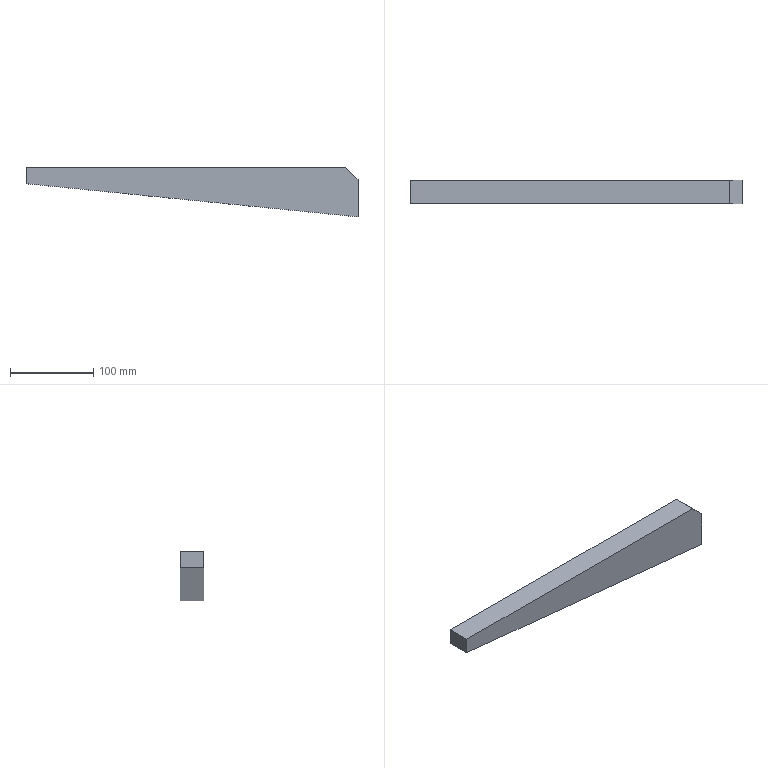Part | SolidWorks | features Extrusion 1 | 1 solid | 7 faces | box 400 x 28 x 60 mm | volume 444850 mm3 | plane 7
STEP:
#1=CARTESIAN_POINT('',(2011.524,0.,-1604.008));
#2=VERTEX_POINT('',#1);
#3=CARTESIAN_POINT('',(2011.524,0.,-1584.008));
#4=VERTEX_POINT('',#3);
#5=CARTESIAN_POINT('',(2011.524,0.,-1604.008));
#6=DIRECTION('',(0.,0.,1.));
#7=VECTOR('',#6,1000.);
#8=LINE('',#5,#7);
#9=EDGE_CURVE('',#2,#4,#8,.T.);
#10=ORIENTED_EDGE('',*,*,#9,.T.);
#11=CARTESIAN_POINT('',(2011.524,28.,-1584.008));
#12=VERTEX_POINT('',#11);
#13=CARTESIAN_POINT('',(2011.524,28.,-1584.008));
#14=DIRECTION('',(0.,-1.,0.));
#15=VECTOR('',#14,1000.);
#16=LINE('',#13,#15);
#17=EDGE_CURVE('',#12,#4,#16,.T.);
#18=ORIENTED_EDGE('',*,*,#17,.F.);
#19=CARTESIAN_POINT('',(2011.524,28.,-1604.008));
#20=VERTEX_POINT('',#19);
#21=CARTESIAN_POINT('',(2011.524,28.,-1604.008));
#22=DIRECTION('',(0.,0.,1.));
#23=VECTOR('',#22,1000.);
#24=LINE('',#21,#23);
#25=EDGE_CURVE('',#20,#12,#24,.T.);
#26=ORIENTED_EDGE('',*,*,#25,.F.);
#27=CARTESIAN_POINT('',(2011.524,28.,-1604.008));
#28=DIRECTION('',(0.,-1.,0.));
#29=VECTOR('',#28,1000.);
#30=LINE('',#27,#29);
#31=EDGE_CURVE('',#20,#2,#30,.T.);
#32=ORIENTED_EDGE('',*,*,#31,.T.);
#33=EDGE_LOOP('',(#10,#18,#26,#32));
#34=FACE_OUTER_BOUND('',#33,.T.);
#35=CARTESIAN_POINT('',(2011.524,28.,-1604.008));
#36=DIRECTION('',(1.,0.,0.));
#37=DIRECTION('',(0.,0.,-1.));
#38=AXIS2_PLACEMENT_3D('',#35,#36,#37);
#39=PLANE('',#38);
#40=ADVANCED_FACE('',(#34),#39,.F.);
#41=CARTESIAN_POINT('',(2396.524,0.,-1584.008));
#42=VERTEX_POINT('',#41);
#43=CARTESIAN_POINT('',(2011.524,0.,-1584.008));
#44=DIRECTION('',(1.,0.,0.));
#45=VECTOR('',#44,1000.);
#46=LINE('',#43,#45);
#47=EDGE_CURVE('',#4,#42,#46,.T.);
#48=ORIENTED_EDGE('',*,*,#47,.T.);
#49=CARTESIAN_POINT('',(2396.524,28.,-1584.008));
#50=VERTEX_POINT('',#49);
#51=CARTESIAN_POINT('',(2396.524,28.,-1584.008));
#52=DIRECTION('',(0.,-1.,0.));
#53=VECTOR('',#52,1000.);
#54=LINE('',#51,#53);
#55=EDGE_CURVE('',#50,#42,#54,.T.);
#56=ORIENTED_EDGE('',*,*,#55,.F.);
#57=CARTESIAN_POINT('',(2011.524,28.,-1584.008));
#58=DIRECTION('',(1.,0.,0.));
#59=VECTOR('',#58,1000.);
#60=LINE('',#57,#59);
#61=EDGE_CURVE('',#12,#50,#60,.T.);
#62=ORIENTED_EDGE('',*,*,#61,.F.);
#63=ORIENTED_EDGE('',*,*,#17,.T.);
#64=EDGE_LOOP('',(#48,#56,#62,#63));
#65=FACE_OUTER_BOUND('',#64,.T.);
#66=CARTESIAN_POINT('',(2011.524,28.,-1584.008));
#67=DIRECTION('',(0.,0.,-1.));
#68=DIRECTION('',(-1.,0.,0.));
#69=AXIS2_PLACEMENT_3D('',#66,#67,#68);
#70=PLANE('',#69);
#71=ADVANCED_FACE('',(#65),#70,.F.);
#72=CARTESIAN_POINT('',(2411.524,0.,-1599.008));
#73=VERTEX_POINT('',#72);
#74=CARTESIAN_POINT('',(2396.524,0.,-1584.008));
#75=DIRECTION('',(0.7071,0.,-0.7071));
#76=VECTOR('',#75,1000.);
#77=LINE('',#74,#76);
#78=EDGE_CURVE('',#42,#73,#77,.T.);
#79=ORIENTED_EDGE('',*,*,#78,.T.);
#80=CARTESIAN_POINT('',(2411.524,28.,-1599.008));
#81=VERTEX_POINT('',#80);
#82=CARTESIAN_POINT('',(2411.524,28.,-1599.008));
#83=DIRECTION('',(0.,-1.,0.));
#84=VECTOR('',#83,1000.);
#85=LINE('',#82,#84);
#86=EDGE_CURVE('',#81,#73,#85,.T.);
#87=ORIENTED_EDGE('',*,*,#86,.F.);
#88=CARTESIAN_POINT('',(2396.524,28.,-1584.008));
#89=DIRECTION('',(0.7071,0.,-0.7071));
#90=VECTOR('',#89,1000.);
#91=LINE('',#88,#90);
#92=EDGE_CURVE('',#50,#81,#91,.T.);
#93=ORIENTED_EDGE('',*,*,#92,.F.);
#94=ORIENTED_EDGE('',*,*,#55,.T.);
#95=EDGE_LOOP('',(#79,#87,#93,#94));
#96=FACE_OUTER_BOUND('',#95,.T.);
#97=CARTESIAN_POINT('',(2396.524,28.,-1584.008));
#98=DIRECTION('',(-0.7071,0.,-0.7071));
#99=DIRECTION('',(-0.7071,0.,0.7071));
#100=AXIS2_PLACEMENT_3D('',#97,#98,#99);
#101=PLANE('',#100);
#102=ADVANCED_FACE('',(#96),#101,.F.);
#103=CARTESIAN_POINT('',(2411.524,0.,-1644.008));
#104=VERTEX_POINT('',#103);
#105=CARTESIAN_POINT('',(2411.524,0.,-1599.008));
#106=DIRECTION('',(0.,0.,-1.));
#107=VECTOR('',#106,1000.);
#108=LINE('',#105,#107);
#109=EDGE_CURVE('',#73,#104,#108,.T.);
#110=ORIENTED_EDGE('',*,*,#109,.T.);
#111=CARTESIAN_POINT('',(2411.524,28.,-1644.008));
#112=VERTEX_POINT('',#111);
#113=CARTESIAN_POINT('',(2411.524,28.,-1644.008));
#114=DIRECTION('',(0.,-1.,0.));
#115=VECTOR('',#114,1000.);
#116=LINE('',#113,#115);
#117=EDGE_CURVE('',#112,#104,#116,.T.);
#118=ORIENTED_EDGE('',*,*,#117,.F.);
#119=CARTESIAN_POINT('',(2411.524,28.,-1599.008));
#120=DIRECTION('',(0.,0.,-1.));
#121=VECTOR('',#120,1000.);
#122=LINE('',#119,#121);
#123=EDGE_CURVE('',#81,#112,#122,.T.);
#124=ORIENTED_EDGE('',*,*,#123,.F.);
#125=ORIENTED_EDGE('',*,*,#86,.T.);
#126=EDGE_LOOP('',(#110,#118,#124,#125));
#127=FACE_OUTER_BOUND('',#126,.T.);
#128=CARTESIAN_POINT('',(2411.524,28.,-1599.008));
#129=DIRECTION('',(-1.,0.,0.));
#130=DIRECTION('',(0.,0.,1.));
#131=AXIS2_PLACEMENT_3D('',#128,#129,#130);
#132=PLANE('',#131);
#133=ADVANCED_FACE('',(#127),#132,.F.);
#134=CARTESIAN_POINT('',(2411.524,0.,-1644.008));
#135=DIRECTION('',(-0.995,0.,0.0995));
#136=VECTOR('',#135,1000.);
#137=LINE('',#134,#136);
#138=EDGE_CURVE('',#104,#2,#137,.T.);
#139=ORIENTED_EDGE('',*,*,#138,.T.);
#140=ORIENTED_EDGE('',*,*,#31,.F.);
#141=CARTESIAN_POINT('',(2411.524,28.,-1644.008));
#142=DIRECTION('',(-0.995,0.,0.0995));
#143=VECTOR('',#142,1000.);
#144=LINE('',#141,#143);
#145=EDGE_CURVE('',#112,#20,#144,.T.);
#146=ORIENTED_EDGE('',*,*,#145,.F.);
#147=ORIENTED_EDGE('',*,*,#117,.T.);
#148=EDGE_LOOP('',(#139,#140,#146,#147));
#149=FACE_OUTER_BOUND('',#148,.T.);
#150=CARTESIAN_POINT('',(2411.524,28.,-1644.008));
#151=DIRECTION('',(0.0995,0.,0.995));
#152=DIRECTION('',(0.995,0.,-0.0995));
#153=AXIS2_PLACEMENT_3D('',#150,#151,#152);
#154=PLANE('',#153);
#155=ADVANCED_FACE('',(#149),#154,.F.);
#156=ORIENTED_EDGE('',*,*,#25,.T.);
#157=ORIENTED_EDGE('',*,*,#61,.T.);
#158=ORIENTED_EDGE('',*,*,#92,.T.);
#159=ORIENTED_EDGE('',*,*,#123,.T.);
#160=ORIENTED_EDGE('',*,*,#145,.T.);
#161=EDGE_LOOP('',(#156,#157,#158,#159,#160));
#162=FACE_OUTER_BOUND('',#161,.T.);
#163=CARTESIAN_POINT('',(0.,28.,0.));
#164=DIRECTION('',(0.,1.,0.));
#165=DIRECTION('',(0.,0.,1.));
#166=AXIS2_PLACEMENT_3D('',#163,#164,#165);
#167=PLANE('',#166);
#168=ADVANCED_FACE('',(#162),#167,.T.);
#169=ORIENTED_EDGE('',*,*,#9,.F.);
#170=ORIENTED_EDGE('',*,*,#138,.F.);
#171=ORIENTED_EDGE('',*,*,#109,.F.);
#172=ORIENTED_EDGE('',*,*,#78,.F.);
#173=ORIENTED_EDGE('',*,*,#47,.F.);
#174=EDGE_LOOP('',(#169,#170,#171,#172,#173));
#175=FACE_OUTER_BOUND('',#174,.T.);
#176=CARTESIAN_POINT('',(0.,0.,0.));
#177=DIRECTION('',(0.,1.,0.));
#178=DIRECTION('',(0.,0.,1.));
#179=AXIS2_PLACEMENT_3D('',#176,#177,#178);
#180=PLANE('',#179);
#181=ADVANCED_FACE('',(#175),#180,.F.);
#182=CLOSED_SHELL('',(#40,#71,#102,#133,#155,#168,#181));
#183=MANIFOLD_SOLID_BREP('',#182);
#184=CARTESIAN_POINT('',(0.,0.,0.));
#185=DIRECTION('',(0.,0.,1.));
#186=DIRECTION('',(1.,0.,0.));
#187=AXIS2_PLACEMENT_3D('',#184,#185,#186);
#188=(LENGTH_UNIT()NAMED_UNIT(*)SI_UNIT(.MILLI.,.METRE.));
#189=UNCERTAINTY_MEASURE_WITH_UNIT(LENGTH_MEASURE(0.00001),#188,'','');
#190=(NAMED_UNIT(*)PLANE_ANGLE_UNIT()SI_UNIT($,.RADIAN.));
#191=(NAMED_UNIT(*)SI_UNIT($,.STERADIAN.)SOLID_ANGLE_UNIT());
#192=(GEOMETRIC_REPRESENTATION_CONTEXT(3)GLOBAL_UNCERTAINTY_ASSIGNED_CONTEXT((#189))GLOBAL_UNIT_ASSIGNED_CONTEXT((#188,#190,#191))REPRESENTATION_CONTEXT('',''));
#193=ADVANCED_BREP_SHAPE_REPRESENTATION('',(#183,#187),#192);